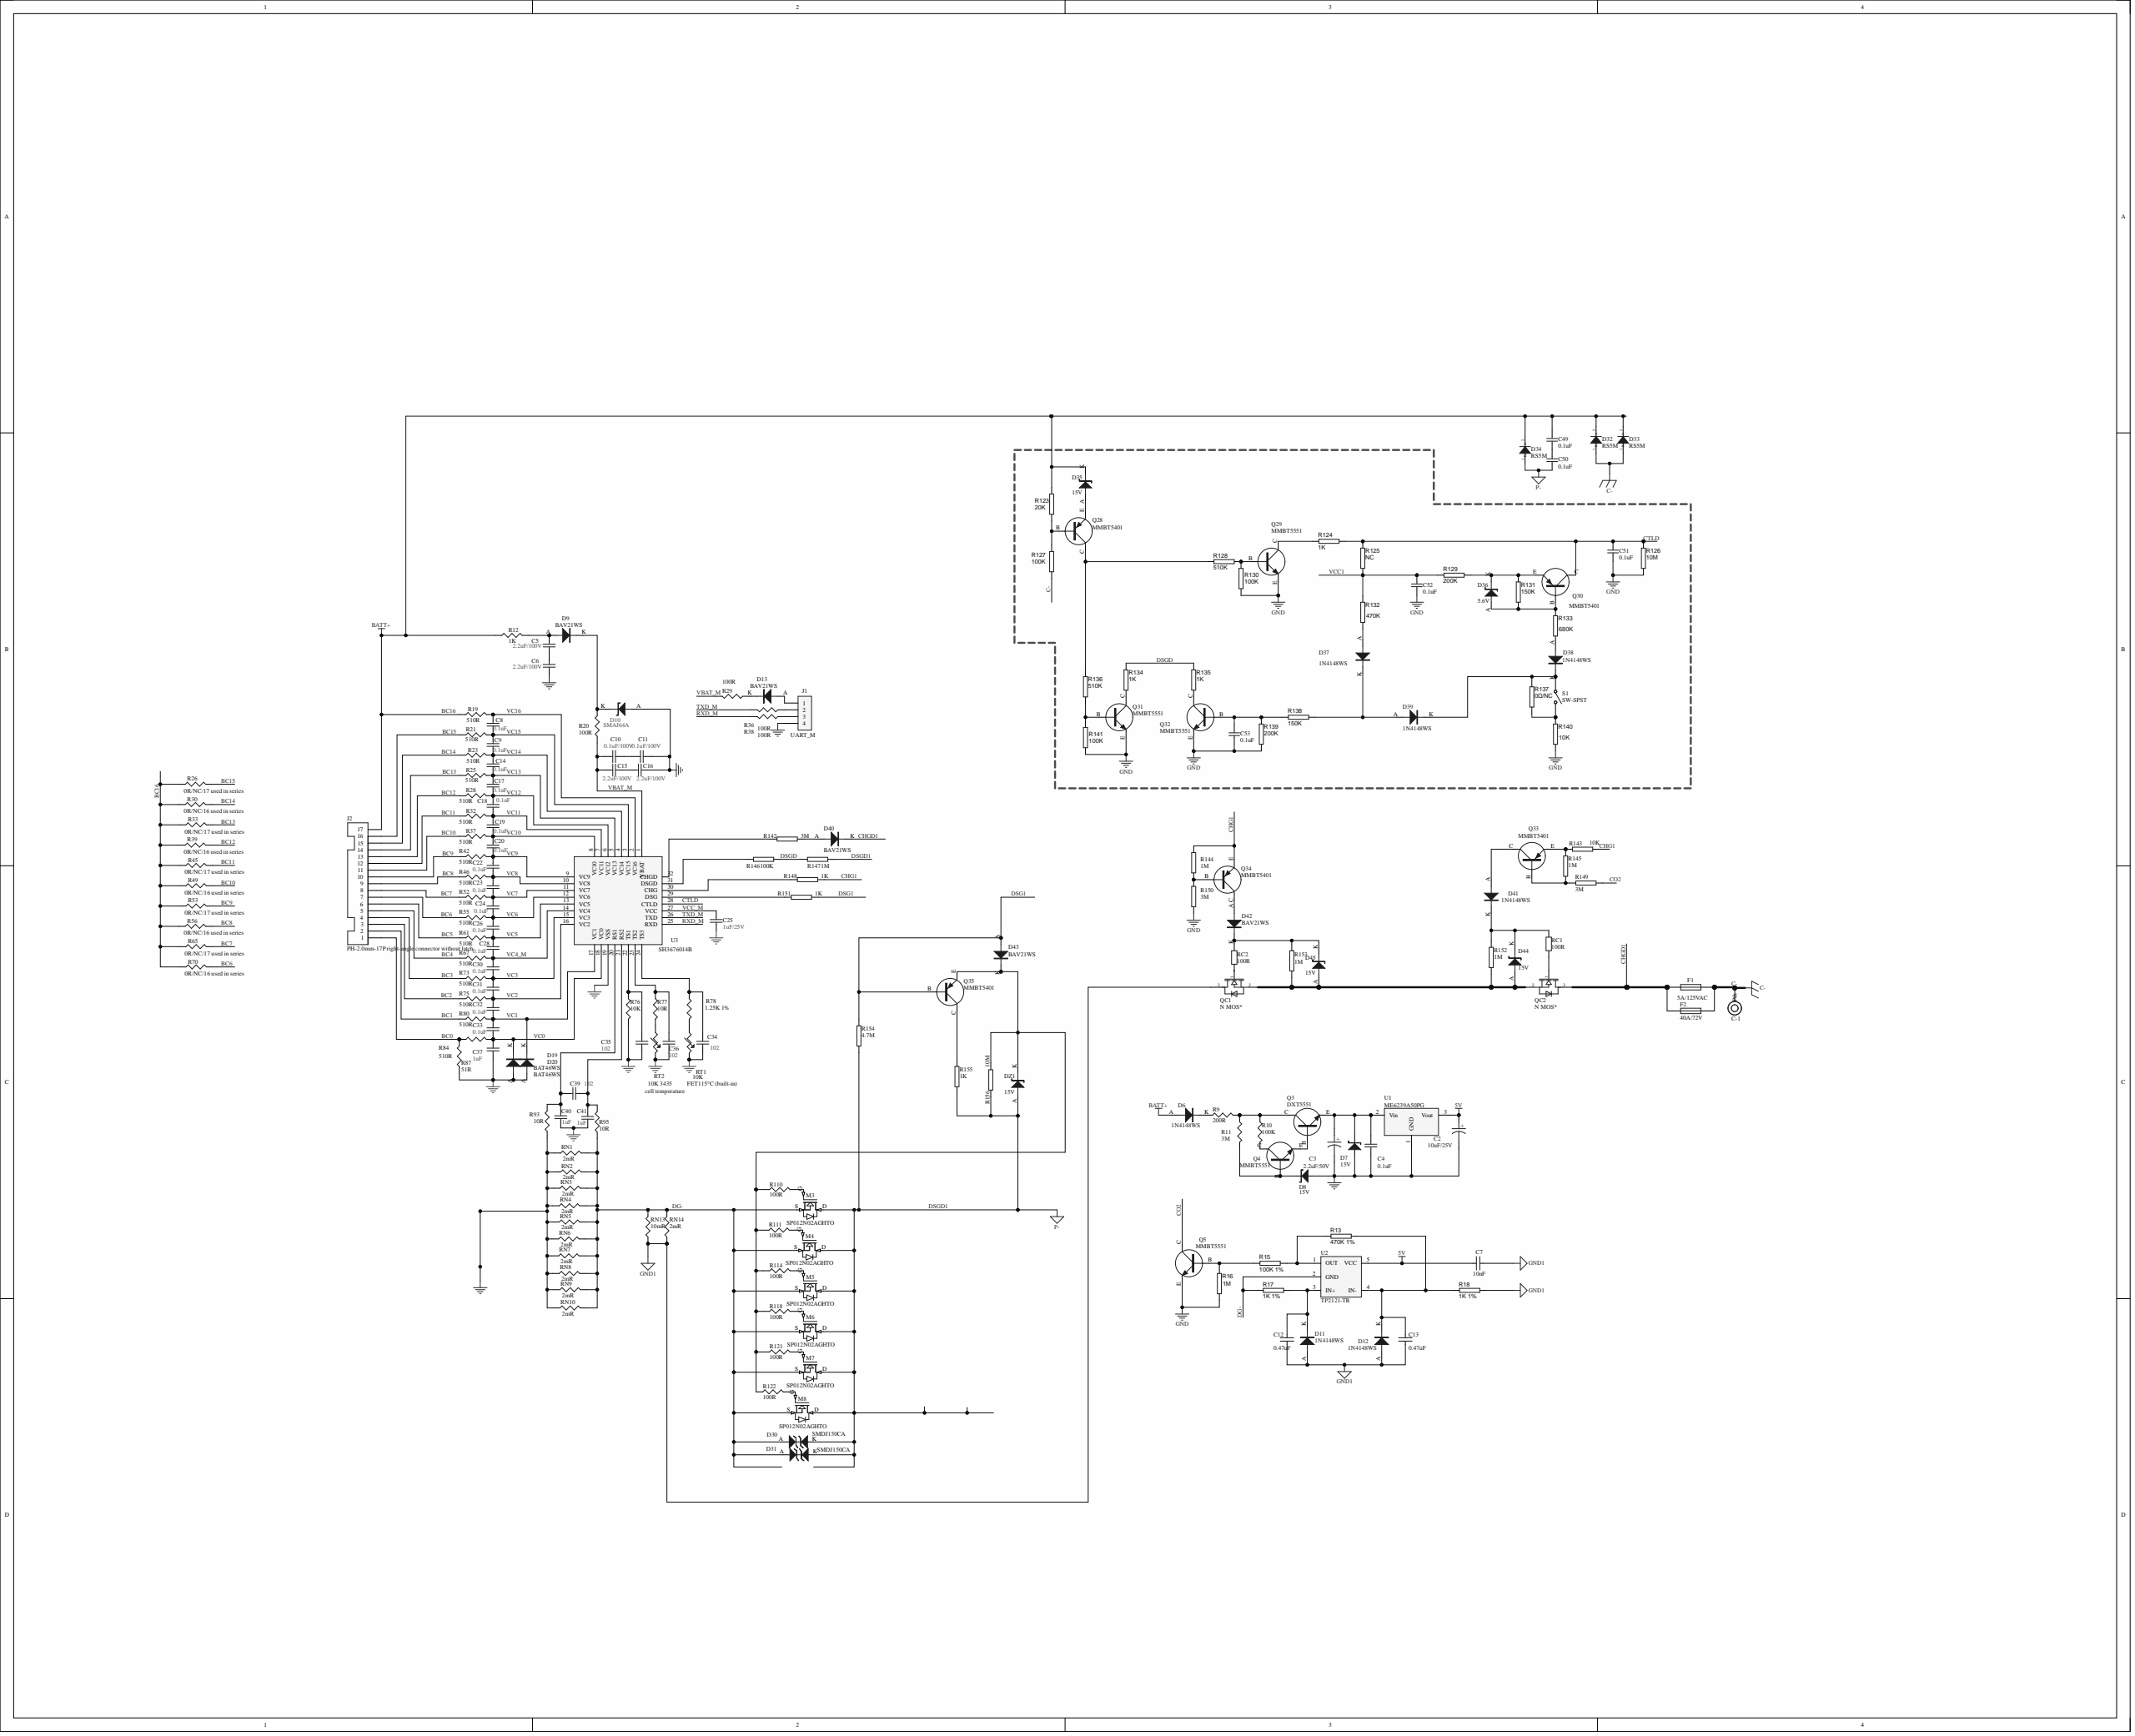Circuit board | Altium Designer | 198 parts | 117 nets
Bill of materials:
Comment,Description,Designator,Footprint,LibRef,Quantity
"10uF/25V","Capacitor","C2","C0805","CAPACITOR POL","1"
"2.2uF/50V","Capacitor","C3","C0805","CAPACITOR POL","1"
"0.1uF","Capacitor","C4, C8, C9, C14, C17, C18, C19, C20, C22, C23, C24, C26, C28, C30, C31, C32, C33","C0603M","CAP","17"
"2.2uF/100V","Capacitor","C5, C6, C15, C16","C0805","CAP","4"
"10nF","CAP","C7","C0603M","CAP","1"
"0.1uF/100V","Capacitor","C10, C11","C0805","CAP","2"
"0.47uF","CAP","C12, C13","C0603M","CAP","2"
"1uF/25V","Capacitor","C25","C0603M","CAP","1"
"102","Capacitor","C34, C35, C36, C39","C0603M","CAP","4"
"1uF","Capacitor","C37, C40, C41","C0603M","CAP","3"
"0.1uF","chip capacitor","C49, C50, C51, C52, C53","C0603A","0805 100nF(104) 10% 50V","5"
"Pth","through-hole pad","C-1","4*3","Pth","1"
"1N4148WS","Diode","D6, D11, D12","SOD-323-E","DIODE","3"
"15V","Zener Diode","D7, D8","SOD-323-E","ZENER2","2"
"BAV21WS","Diode","D9, D13","SOD-323-E","DIODE","2"
"SMAJ64A","Zener Diode","D10","SMA","ZENER2","1"
"BAT46WS","Diode","D19, D20","SOD-323-E","DIODE","2"
"SMDJ150CA","bidirectional ESD","D30, D31","SMC-BI","diode-esd","2"
"RS5M","chip diode","D32, D33, D34","SMC_MDO-214AB)","RS5M","3"
"15V","Zener Diode","D35, D44, D45, DZ1","SOD323(A+K-)","ZENER2","4"
"5.6V","Zener Diode","D36","SOD323(A+K-)","ZENER2","1"
"1N4148WS","Diode","D37, D38, D39, D41","SOD323(A+K-)","DIODE","4"
"BAV21WS","Diode","D40, D42, D43","SOD323(A+K-)","DIODE","3"
"5A/125VAC","Fuse","F1","R1206L","FUSE1","1"
"40A/72V","Fuse","F2","R1206L","FUSE1","1"
"UART_M","Connector","J1","CON4/2.0","CON4","1"
"PH-2.0mm-17P right-angle connector without latch","PH-2.0mm-17P right-angle connector without latch","J2","HY2.0WT-17A/P 卧贴带扣耐温260℃","PH-2.0mm-17P弯脚不带扣","1"
"SP012N02AGHTO","","M3, M4, M5, M6, M7, M8","TOLL","MOSFET N","6"
"DXT5551","NPN Transistor","Q3","SOT-89BCE","NPN","1"
"MMBT5551","NPN Transistor","Q4, Q5","SOT-23S","NPN","2"
"MMBT5401","PNP Transistor","Q28, Q30, Q33, Q34, Q35","SOT23-3_BEC","PNP","5"
"MMBT5551","NPN Transistor","Q29, Q31, Q32","SOT23-3_BEC","NPN","3"
"N MOS*","chip MOS","QC1, QC2","TOLL","N MOS*","2"
"200R","","R9","R0805","RES1","1"
"100K","","R10","R0603m","RES1","1"
"3M","","R11","R0603m","RES1","1"
"1K","","R12","R0805","RES1","1"
"470K 1%","RES","R13","R0603m","RES1","1"
"100K 1%","RES","R15","R0603m","RES1","1"
"1M","RES","R16","R0603m","RES1","1"
"1K 1%","RES","R17, R18","R0603m","RES1","2"
"510R","","R19, R21, R23, R25, R28, R32, R37, R42, R46, R52, R55, R61, R67, R73, R75, R80, R84","R0603m","RES1","17"
"100R","","R20","R0805","RES1","1"
"0R/NC/17 used in series","","R26, R33, R45, R53, R65","R0805A","RES1","5"
"100R","","R29, R36, R38, R110, R111, R114, R118, R121, R122","R0603m","RES1","9"
"0R/NC/16 used in series","","R30, R39, R49, R56, R70","R0805A","RES1","5"
"10K","","R76","R0603m","RES1","1"
"10R","","R77, R93, R95","R0603m","RES1","3"
"1.25K 1%","","R78","R0603m","RES1","1"
"51R","","R87","R0805","RES1","1"
"20K","RES","R123","R0603A","RES1","1"
"1K","RES","R124, R134, R135, R148, R151, R155","R0603A","RES1","6"
"NC","RES","R125","R0603A","RES1","1"
"10M","RES","R126, R156","R0603A","RES1","2"
"100K","RES","R127, R130, R141, R146","R0603A","RES1","4"
"510K","RES","R128, R136","R0603A","RES1","2"
"200K","RES","R129, R139","R0603A","RES1","2"
"150K","RES","R131, R138","R0603A","RES1","2"
"470K","RES","R132","R0603A","RES1","1"
"680K","RES","R133","R0603A","RES1","1"
"0Ω/NC","RES","R137","R0603A","RES1","1"
"10K","RES, [NoValue]","R140, R143","R0603A","RES1, RES","2"
"3M","RES, [NoValue]","R142, R149, R150","R0603A","RES1, RES","3"
"1M","RES, [NoValue]","R144, R145, R147, R152, R153","R0603A","RES1, RES","5"
"4.7M","RES","R154","R0603A","RES1","1"
"100R","chip resistor","RC1, RC2","R0603A","0603 1.2MΩ (1204) 1%","2"
"2mR","","RN1, RN2, RN3, RN4, RN5, RN6, RN7, RN8, RN9, RN10, RN14","R2512A","RES1","11"
"10mR","","RN13","R2512A","RES1","1"
"10K","","RT1","R0603","RES3","1"
"10K 3435","","RT2","NTC-DIP","RES3","1"
"SW-SPST","Single-Pole, Single-Throw Switch","S1","NTC-DIP","SW-SPST","1"
"ME6239A50PG","","U1","SO-89","VOLTREG","1"
"TP2121-TR","S8211D","U2","SOT23-5","TP2121-TR","1"
"SH3676014B","","U3","LQFP-32","SH3676016B","1"
Netlist (Protel format):
[
C2
C0805
10uF/25V



]
[
C3
C0805
2.2uF/50V



]
[
C4
C0603M
0.1uF



]
[
C5
C0805
2.2uF/100V



]
[
C6
C0805
2.2uF/100V



]
[
C7
C0603M
10nF



]
[
C8
C0603M
0.1uF



]
[
C9
C0603M
0.1uF



]
[
C10
C0805
0.1uF/100V



]
[
C11
C0805
0.1uF/100V



]
[
C12
C0603M
0.47uF



]
[
C13
C0603M
0.47uF



]
[
C14
C0603M
0.1uF



]
[
C15
C0805
2.2uF/100V



]
[
C16
C0805
2.2uF/100V



]
[
C17
C0603M
0.1uF



]
[
C18
C0603M
0.1uF



]
[
C19
C0603M
0.1uF



]
[
C20
C0603M
0.1uF



]
[
C22
C0603M
0.1uF



]
[
C23
C0603M
0.1uF



]
[
C24
C0603M
0.1uF



]
[
C25
C0603M
1uF/25V



]
[
C26
C0603M
0.1uF



]
[
C28
C0603M
0.1uF



]
[
C30
C0603M
0.1uF



]
[
C31
C0603M
0.1uF



]
[
C32
C0603M
0.1uF



]
[
C33
C0603M
0.1uF



]
[
C34
C0603M
102



]
[
C35
C0603M
102



]
[
C36
C0603M
102



]
[
C37
C0603M
1uF



]
[
C39
C0603M
102



]
[
C40
C0603M
1uF



]
[
C41
C0603M
1uF



]
[
C49
C0603A
0.1uF



]
[
C50
C0603A
0.1uF



]
[
C51
C0603A
0.1uF



]
[
C52
C0603A
0.1uF



]
[
C53
C0603A
0.1uF



]
[
C-1
4*3
Pth



]
[
D6
SOD-323-E
1N4148WS



]
[
D7
SOD-323-E
15V



]
[
D8
SOD-323-E
15V



]
[
D9
SOD-323-E
BAV21WS



]
[
D10
SMA
SMAJ64A



]
[
D11
SOD-323-E
1N4148WS



]
[
D12
SOD-323-E
1N4148WS



]
[
D13
SOD-323-E
BAV21WS



]
[
D19
SOD-323-E
BAT46WS



]
[
D20
SOD-323-E
BAT46WS



]
[
D30
SMC-BI
SMDJ150CA



]
[
D31
SMC-BI
SMDJ150CA



]
[
D32
SMC_MDO-214AB)
RS5M



]
[
D33
SMC_MDO-214AB)
RS5M



]
[
D34
SMC_MDO-214AB)
RS5M



]
[
D35
SOD323(A+K-)
15V



]
[
D36
SOD323(A+K-)
5.6V



]
[
D37
SOD323(A+K-)
1N4148WS



]
[
D38
SOD323(A+K-)
1N4148WS



]
[
D39
SOD323(A+K-)
1N4148WS



]
[
D40
SOD323(A+K-)
BAV21WS



]
[
D41
SOD323(A+K-)
1N4148WS



]
[
D42
SOD323(A+K-)
BAV21WS



]
[
D43
SOD323(A+K-)
BAV21WS



]
[
D44
SOD323(A+K-)
15V



]
[
D45
SOD323(A+K-)
15V



]
[
DZ1
SOD323(A+K-)
15V



]
[
F1
R1206L
5A/125VAC



]
[
F2
R1206L
40A/72V



]
[
J1
CON4/2.0
UART_M



]
[
J2
HY2.0WT-17A/P 卧贴带扣耐温260℃
PH-2.0mm-17P right-angle connector without latch



]
[
M3
TOLL
SP012N02AGHTO



]
[
M4
TOLL
SP012N02AGHTO



]
[
M5
TOLL
SP012N02AGHTO



]
[
M6
TOLL
SP012N02AGHTO



]
[
M7
TOLL
SP012N02AGHTO



]
[
M8
TOLL
SP012N02AGHTO



]
[
Q3
SOT-89BCE
DXT5551



]
[
Q4
SOT-23S
MMBT5551



]
[
Q5
SOT-23S
MMBT5551



]
[
Q28
SOT23-3_BEC
MMBT5401



]
[
Q29
SOT23-3_BEC
MMBT5551



]
[
Q30
SOT23-3_BEC
MMBT5401



]
[
Q31
SOT23-3_BEC
MMBT5551



]
[
Q32
SOT23-3_BEC
MMBT5551



]
[
Q33
SOT23-3_BEC
MMBT5401



]
[
Q34
SOT23-3_BEC
MMBT5401



]
[
Q35
SOT23-3_BEC
MMBT5401



]
[
QC1
TOLL
N MOS*



]
[
QC2
TOLL
N MOS*



]
[
R9
R0805
200R



]
[
R10
R0603m
100K



]
[
R11
R0603m
3M



]
[
R12
R0805
1K



]
[
R13
R0603m
470K 1%



]
[
R15
R0603m
100K 1%



]
[
R16
R0603m
1M



]
[
R17
R0603m
1K 1%



]
[
R18
R0603m
1K 1%



]
[
R19
R0603m
510R



]
[
R20
R0805
100R



]
[
R21
R0603m
510R



]
[
R23
R0603m
510R



]
[
R25
R0603m
510R



]
[
R26
R0805A
0R/NC/17 used in series



]
[
R28
R0603m
510R



]
[
R29
R0603m
100R



]
[
R30
R0805A
0R/NC/16 used in series



]
[
R32
R0603m
510R



]
[
R33
R0805A
0R/NC/17 used in series



]
[
R36
R0603m
100R



]
[
R37
R0603m
510R



]
[
R38
R0603m
100R



]
[
R39
R0805A
0R/NC/16 used in series



]
[
R42
R0603m
510R



]
[
R45
R0805A
0R/NC/17 used in series



]
[
R46
R0603m
510R



]
[
R49
R0805A
0R/NC/16 used in series



]
[
R52
R0603m
510R



]
[
R53
R0805A
0R/NC/17 used in series



]
[
R55
R0603m
510R



]
[
R56
R0805A
0R/NC/16 used in series



]
[
R61
R0603m
510R



]
[
R65
R0805A
0R/NC/17 used in series



]
[
R67
R0603m
510R



]
[
R70
R0805A
0R/NC/16 used in series



]
[
R73
R0603m
510R



]
[
R75
R0603m
510R



]
[
R76
R0603m
10K



]
[
R77
R0603m
10R



]
[
R78
R0603m
1.25K 1%



]
[
R80
R0603m
510R



]
[
R84
R0603m
510R



]
[
R87
R0805
51R



]
[
R93
R0603m
10R



]
[
R95
R0603m
10R



]
[
R110
R0603m
100R



]
[
R111
R0603m
100R



]
[
R114
R0603m
100R



]
[
R118
R0603m
100R



]
[
R121
R0603m
100R



]
[
R122
R0603m
100R



]
[
R123
R0603A
20K



]
[
R124
R0603A
1K



]
[
R125
R0603A
NC



]
[
R126
R0603A
10M



]
[
R127
R0603A
100K



]
[
R128
R0603A
510K



]
[
R129
R0603A
200K



]
[
R130
R0603A
100K



]
[
R131
R0603A
150K



]
[
R132
R0603A
470K



]
[
R133
R0603A
680K



]
[
R134
R0603A
1K



]
[
R135
R0603A
1K



]
[
R136
R0603A
510K



]
[
R137
R0603A
0Ω/NC



]
[
R138
R0603A
150K



]
[
R139
R0603A
200K



]
[
R140
R0603A
10K



]
[
R141
R0603A
100K



]
[
R142
R0603A
3M



]
[
R143
R0603A
10K



]
[
R144
R0603A
1M



]
[
R145
R0603A
1M



]
[
R146
R0603A
100K



]
[
R147
R0603A
1M



]
[
R148
R0603A
1K



]
[
R149
R0603A
3M



]
[
R150
R0603A
3M



]
[
R151
R0603A
1K



]
[
R152
R0603A
1M



]
[
R153
R0603A
1M



]
[
R154
R0603A
4.7M



]
[
R155
R0603A
1K



]
[
R156
R0603A
10M



]
[
RC1
R0603A
100R



]
[
RC2
R0603A
100R



]
[
RN1
R2512A
2mR



]
[
RN2
R2512A
2mR



]
[
RN3
R2512A
2mR



]
[
RN4
R2512A
2mR



]
[
RN5
R2512A
2mR



]
[
RN6
R2512A
2mR



]
[
RN7
R2512A
2mR



]
[
RN8
R2512A
2mR



]
[
RN9
R2512A
2mR



]
[
RN10
R2512A
2mR



]
[
RN13
R2512A
10mR



]
[
RN14
R2512A
2mR



]
[
RT1
R0603
10K



]
[
RT2
NTC-DIP
10K 3435



]
[
S1
NTC-DIP
SW-SPST



]
[
U1
SO-89
ME6239A50PG



]
[
U2
SOT23-5
TP2121-TR



]
[
U3
LQFP-32
SH3676014B



]
(
VCC_M
C25-1
U3-27
)
(
VCC1
C52-2
R125-2
R129-2
R132-1
)
(
VC16
C8-1
R19-2
U3-2
)
(
VC15
C8-2
C9-1
R21-2
U3-3
)
(
VC14
C9-2
C14-1
R23-2
U3-4
)
(
VC13
C14-2
C17-1
R25-2
U3-5
)
(
VC12
C17-2
C18-1
R28-2
U3-6
)
(
VC11
C18-2
C19-1
R32-2
U3-7
)
(
VC10
C19-2
C20-1
R37-2
U3-8
)
(
VC9
C20-2
C22-1
R42-2
U3-9
)
(
VC8
C22-2
C23-1
R46-2
U3-10
)
(
VC7
C23-2
C24-1
R52-2
U3-11
)
(
VC6
C24-2
C26-1
R55-2
U3-12
)
(
VC5
C26-2
C28-1
R61-2
U3-13
)
(
VC4_M
C28-2
C30-1
R67-2
U3-14
)
(
VC3
C30-2
C31-1
R73-2
U3-15
)
(
VC2
C31-2
C32-1
R75-2
U3-16
)
(
VC1
C32-2
C33-1
D19-K
R80-2
U3-17
)
(
VC0
C33-2
C37-1
D20-K
R84-2
U3-18
)
(
VBAT_M
C10-1
C15-1
R20-1
R29-2
U3-1
)
(
TXD_M
R38-2
U3-26
)
(
RXD_M
R36-2
U3-25
)
(
NetR151_2
R151-2
U3-29
)
(
NetR148_2
R148-2
U3-30
)
(
NetR146_2
R146-2
U3-31
)
(
NetR142_2
R142-2
U3-32
)
(
NetR137_2
R137-2
R140-1
S1-2
)
(
NetR78_2
R78-2
RT1-1
)
(
NetR77_2
R77-2
RT2-1
)
(
NetR13_2
R13-2
R15-1
U2-1
)
(
NetQC2_1
QC2-1
RC1-2
)
(
NetQC1_1
QC1-1
RC2-1
)
(
NetQ35_C
Q35-C
R155-1
)
(
NetQ34_B
Q34-B
R144-1
R150-1
)
(
NetQ33_E
Q33-E
R143-1
R145-2
)
(
NetQ33_B
Q33-B
R145-1
R149-2
)
(
NetQ32_C
Q32-C
R135-1
)
(
NetQ31_C
Q31-C
R134-1
)
(
NetQ31_B
Q31-B
R136-1
R141-2
)
(
NetQ29_C
Q29-C
R124-1
)
(
NetQ29_B
Q29-B
R128-1
R130-2
)
(
NetQ28_C
Q28-C
R128-2
R136-2
)
(
NetQ28_B
Q28-B
R123-1
R127-2
)
(
NetQ5_B
Q5-B
R15-2
R16-2
)
(
NetQ4_C
Q4-C
R10-2
)
(
NetQ3_C
Q3-C
R9-1
R10-1
R11-1
)
(
NetQ3_B
Q3-B
Q4-E
)
(
NetM8_G
M8-G
R122-2
)
(
NetM7_G
M7-G
R121-2
)
(
NetM6_G
M6-G
R118-2
)
(
NetM5_G
M5-G
R114-2
)
(
NetM4_G
M4-G
R111-2
)
(
NetM3_G
M3-G
R110-2
)
(
NetJ1_3
J1-3
R36-1
)
(
NetJ1_2
J1-2
R38-1
)
(
NetD44_A
D44-A
D45-A
QC1-2
QC2-2
R152-2
R153-1
)
(
NetD43_K
D43-K
DZ1-K
Q35-E
R110-1
R111-1
R114-1
R118-1
R121-1
R122-1
R156-2
)
(
NetD42_K
D42-K
D45-K
R153-2
RC2-2
)
(
NetD42_A
D42-A
Q34-C
)
(
NetD41_K
D41-K
D44-K
R152-1
RC1-1
)
(
NetD41_A
D41-A
Q33-C
)
(
NetD40_A
D40-A
R142-1
)
(
NetD38_K
D38-K
D39-K
R137-1
S1-1
)
(
NetD38_A
D38-A
R133-2
)
(
NetD37_K
D37-K
D39-A
R138-2
)
(
NetD37_A
D37-A
R132-2
)
(
NetD36_K
D36-K
Q30-E
R129-1
R131-2
)
(
NetD36_A
D36-A
Q30-B
R131-1
R133-1
)
(
NetD35_A
D35-A
Q28-E
)
(
NetD13_K
D13-K
R29-1
)
(
NetD13_A
D13-A
J1-1
)
(
NetD9_K
D9-K
D10-K
R20-2
)
(
NetD8_K
D8-K
Q4-B
R11-2
)
(
NetD6_K
D6-K
R9-2
)
(
NetC53_2
C53-2
Q32-B
R138-1
R139-2
)
(
NetC49_1
C49-1
C50-2
)
(
NetC39_2
C39-2
C40-1
R93-2
U3-20
)
(
NetC39_1
C39-1
C41-1
R95-2
U3-21
)
(
NetC36_2
C36-2
R77-1
U3-23
)
(
NetC35_2
C35-2
R76-1
U3-22
)
(
NetC34_2
C34-2
R78-1
U3-24
)
(
NetC15_2
C15-2
C16-1
)
(
NetC13_1
C13-1
D12-K
R13-1
R18-2
U2-4
)
(
NetC12_1
C12-1
D11-K
R17-1
U2-3
)
(
NetC10_2
C10-2
C11-1
)
(
NetC5_2
C5-2
D9-A
R12-2
)
(
NetC5_1
C5-1
C6-2
)
(
NetC3_1
C3-1
C4-1
D7-K
Q3-E
U1-2
)
(
GND1
C7-2
C12-2
C13-2
D11-A
D12-A
QC1-3
R18-1
RN13-1
RN14-1
)
(
GND
C2-2
C3-2
C4-2
C6-1
C11-2
C16-2
C25-2
C34-1
C35-1
C36-1
C37-2
C40-2
C41-2
C51-1
C52-1
C53-1
D7-A
D8-A
D10-A
D19-A
D20-A
J1-4
Q5-E
Q29-E
Q31-E
Q32-E
R16-1
R76-2
R87-1
R93-1
R126-1
R130-1
R139-1
R140-2
R141-1
R150-2
RN1-1
RN2-1
RN3-1
RN4-1
RN5-1
RN6-1
RN7-1
RN8-1
RN9-1
RN10-1
RT1-2
RT2-2
U1-1
U3-19
)
(
DSGD1
C50-1
D30-K
D31-K
D34-1
DZ1-A
M3-D
M4-D
M5-D
M6-D
M7-D
M8-D
R147-1
R154-1
R155-2
R156-1
)
(
DSGD
R134-2
R135-2
R146-1
R147-2
)
(
DSG1
D43-A
Q35-B
R151-1
R154-2
)
(
DG-
D30-A
D31-A
M3-S
M4-S
M5-S
M6-S
M7-S
M8-S
R17-2
R95-1
RN1-2
RN2-2
RN3-2
RN4-2
RN5-2
RN6-2
RN7-2
RN8-2
RN9-2
RN10-2
RN13-2
RN14-2
U2-2
)
(
CTLD
C51-2
Q30-C
R124-2
R125-1
R126-2
U3-28
)
(
CO2
Q5-C
R149-1
)
(
CHGD1
D40-K
F1-1
F2-1
QC2-3
)
(
CHG1
Q34-E
R143-2
R144-2
R148-1
)
(
C-
C-1-1
D32-1
D33-1
F1-2
F2-2
R127-1
)
(
BC16
C49-2
D6-A
D32-2
D33-2
D34-2
D35-K
J2-17
R12-1
R19-1
R26-1
R30-1
R33-1
R39-1
R45-1
R49-1
R53-1
R56-1
R65-1
R70-1
R123-2
)
(
BC15
J2-16
R21-1
R26-2
)
(
BC14
J2-15
R23-1
R30-2
)
(
BC13
J2-14
R25-1
R33-2
)
(
BC12
J2-13
R28-1
R39-2
)
(
BC11
J2-12
R32-1
R45-2
)
(
BC10
J2-11
R37-1
R49-2
)
(
BC9
J2-10
R42-1
R53-2
)
(
BC8
J2-9
R46-1
R56-2
)
(
BC7
J2-8
R52-1
R65-2
)
(
BC6
J2-7
R55-1
R70-2
)
(
BC5
J2-6
R61-1
)
(
BC4
J2-5
R67-1
)
(
BC3
J2-4
R73-1
)
(
BC2
J2-3
R75-1
)
(
BC1
J2-2
R80-1
)
(
BC0
J2-1
R84-1
R87-2
)
(
5V
C2-1
C7-1
U1-3
U2-5
)